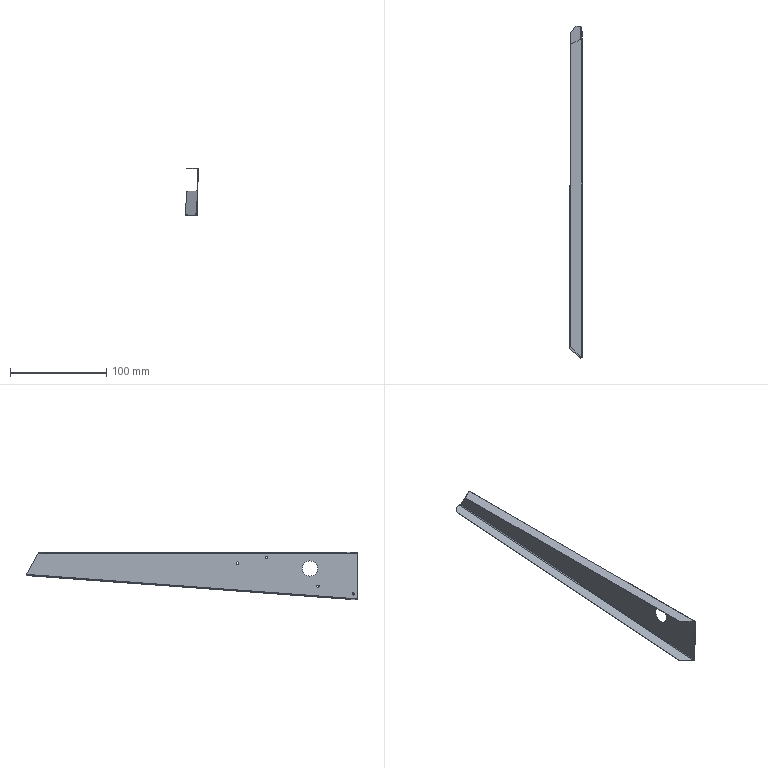Part | SolidWorks | features BaseBody 1 | 1 solid | 35 faces | box 13.154 x 345.624 x 49.869 mm | volume 9893 mm3 | plane 15 | cylinder 14 | spline 6 | commonest cylinder face diameters 2.4 x8 1.473 x2 2.473 x2 15.9 x2
STEP:
#1=CARTESIAN_POINT('',(-0.6458,-122.,-25.162));
#2=VERTEX_POINT('',#1);
#3=CARTESIAN_POINT('',(-0.2296,-122.,-9.267));
#4=VERTEX_POINT('',#3);
#5=CARTESIAN_POINT('',(-0.4377,-122.,-17.214));
#6=DIRECTION('',(-0.9997,0.,0.02618));
#7=DIRECTION('',(-0.02618,0.,-0.9997));
#8=AXIS2_PLACEMENT_3D('',#5,#6,#7);
#9=CIRCLE('',#8,7.95);
#10=EDGE_CURVE('',#2,#4,#9,.T.);
#11=ORIENTED_EDGE('',*,*,#10,.T.);
#12=CARTESIAN_POINT('',(0.2703,-122.,-9.28));
#13=VERTEX_POINT('',#12);
#14=CARTESIAN_POINT('',(-0.2296,-122.,-9.267));
#15=DIRECTION('',(0.9997,0.,-0.02618));
#16=VECTOR('',#15,1000.);
#17=LINE('',#14,#16);
#18=EDGE_CURVE('',#4,#13,#17,.T.);
#19=ORIENTED_EDGE('',*,*,#18,.T.);
#20=CARTESIAN_POINT('',(-0.146,-122.,-25.175));
#21=VERTEX_POINT('',#20);
#22=CARTESIAN_POINT('',(0.06215,-122.,-17.227));
#23=DIRECTION('',(0.9997,0.,-0.02618));
#24=DIRECTION('',(-0.02618,0.,-0.9997));
#25=AXIS2_PLACEMENT_3D('',#22,#23,#24);
#26=CIRCLE('',#25,7.95);
#27=EDGE_CURVE('',#13,#21,#26,.T.);
#28=ORIENTED_EDGE('',*,*,#27,.T.);
#29=CARTESIAN_POINT('',(-0.6458,-122.,-25.162));
#30=DIRECTION('',(0.9997,0.,-0.02618));
#31=VECTOR('',#30,1000.);
#32=LINE('',#29,#31);
#33=EDGE_CURVE('',#2,#21,#32,.T.);
#34=ORIENTED_EDGE('',*,*,#33,.F.);
#35=EDGE_LOOP('',(#11,#19,#28,#34));
#36=FACE_OUTER_BOUND('',#35,.T.);
#37=CARTESIAN_POINT('',(-0.4377,-122.,-17.214));
#38=DIRECTION('',(0.9997,0.,-0.02618));
#39=DIRECTION('',(-0.02618,0.,-0.9997));
#40=AXIS2_PLACEMENT_3D('',#37,#38,#39);
#41=CYLINDRICAL_SURFACE('',#40,7.95);
#42=ADVANCED_FACE('',(#36),#41,.F.);
#43=CARTESIAN_POINT('',(-0.3859,-130.324,-34.336));
#44=VERTEX_POINT('',#43);
#45=CARTESIAN_POINT('',(-0.4487,-130.324,-36.736));
#46=VERTEX_POINT('',#45);
#47=CARTESIAN_POINT('',(-0.4173,-130.324,-35.536));
#48=DIRECTION('',(0.9997,0.,-0.02618));
#49=DIRECTION('',(0.02618,0.,0.9997));
#50=AXIS2_PLACEMENT_3D('',#47,#48,#49);
#51=CIRCLE('',#50,1.2);
#52=EDGE_CURVE('',#44,#46,#51,.T.);
#53=ORIENTED_EDGE('',*,*,#52,.T.);
#54=CARTESIAN_POINT('',(-0.9485,-130.324,-36.723));
#55=VERTEX_POINT('',#54);
#56=CARTESIAN_POINT('',(-0.4487,-130.324,-36.736));
#57=DIRECTION('',(-0.9997,0.,0.02618));
#58=VECTOR('',#57,1000.);
#59=LINE('',#56,#58);
#60=EDGE_CURVE('',#46,#55,#59,.T.);
#61=ORIENTED_EDGE('',*,*,#60,.T.);
#62=CARTESIAN_POINT('',(-0.8857,-130.324,-34.323));
#63=VERTEX_POINT('',#62);
#64=CARTESIAN_POINT('',(-0.9171,-130.324,-35.523));
#65=DIRECTION('',(0.9997,0.,-0.02618));
#66=DIRECTION('',(0.02618,0.,0.9997));
#67=AXIS2_PLACEMENT_3D('',#64,#65,#66);
#68=CIRCLE('',#67,1.2);
#69=EDGE_CURVE('',#63,#55,#68,.T.);
#70=ORIENTED_EDGE('',*,*,#69,.F.);
#71=CARTESIAN_POINT('',(-0.3859,-130.324,-34.336));
#72=DIRECTION('',(-0.9997,0.,0.02618));
#73=VECTOR('',#72,1000.);
#74=LINE('',#71,#73);
#75=EDGE_CURVE('',#44,#63,#74,.T.);
#76=ORIENTED_EDGE('',*,*,#75,.F.);
#77=EDGE_LOOP('',(#53,#61,#70,#76));
#78=FACE_OUTER_BOUND('',#77,.T.);
#79=CARTESIAN_POINT('',(-0.4173,-130.324,-35.536));
#80=DIRECTION('',(-0.9997,0.,0.02618));
#81=DIRECTION('',(0.02618,0.,0.9997));
#82=AXIS2_PLACEMENT_3D('',#79,#80,#81);
#83=CYLINDRICAL_SURFACE('',#82,1.2);
#84=ADVANCED_FACE('',(#78),#83,.F.);
#85=CARTESIAN_POINT('',(-0.5954,-167.,-42.338));
#86=VERTEX_POINT('',#85);
#87=CARTESIAN_POINT('',(-0.6582,-167.,-44.738));
#88=VERTEX_POINT('',#87);
#89=CARTESIAN_POINT('',(-0.6268,-167.,-43.538));
#90=DIRECTION('',(0.9997,0.,-0.02618));
#91=DIRECTION('',(0.02618,0.,0.9997));
#92=AXIS2_PLACEMENT_3D('',#89,#90,#91);
#93=CIRCLE('',#92,1.2);
#94=EDGE_CURVE('',#86,#88,#93,.T.);
#95=ORIENTED_EDGE('',*,*,#94,.T.);
#96=CARTESIAN_POINT('',(-1.158,-167.,-44.724));
#97=VERTEX_POINT('',#96);
#98=CARTESIAN_POINT('',(-0.6582,-167.,-44.738));
#99=DIRECTION('',(-0.9997,0.,0.02618));
#100=VECTOR('',#99,1000.);
#101=LINE('',#98,#100);
#102=EDGE_CURVE('',#88,#97,#101,.T.);
#103=ORIENTED_EDGE('',*,*,#102,.T.);
#104=CARTESIAN_POINT('',(-1.095,-167.,-42.325));
#105=VERTEX_POINT('',#104);
#106=CARTESIAN_POINT('',(-1.127,-167.,-43.525));
#107=DIRECTION('',(0.9997,0.,-0.02618));
#108=DIRECTION('',(0.02618,0.,0.9997));
#109=AXIS2_PLACEMENT_3D('',#106,#107,#108);
#110=CIRCLE('',#109,1.2);
#111=EDGE_CURVE('',#105,#97,#110,.T.);
#112=ORIENTED_EDGE('',*,*,#111,.F.);
#113=CARTESIAN_POINT('',(-0.5954,-167.,-42.338));
#114=DIRECTION('',(-0.9997,0.,0.02618));
#115=VECTOR('',#114,1000.);
#116=LINE('',#113,#115);
#117=EDGE_CURVE('',#86,#105,#116,.T.);
#118=ORIENTED_EDGE('',*,*,#117,.F.);
#119=EDGE_LOOP('',(#95,#103,#112,#118));
#120=FACE_OUTER_BOUND('',#119,.T.);
#121=CARTESIAN_POINT('',(-0.6268,-167.,-43.538));
#122=DIRECTION('',(-0.9997,0.,0.02618));
#123=DIRECTION('',(0.02618,0.,0.9997));
#124=AXIS2_PLACEMENT_3D('',#121,#122,#123);
#125=CYLINDRICAL_SURFACE('',#124,1.2);
#126=ADVANCED_FACE('',(#120),#125,.F.);
#127=CARTESIAN_POINT('',(0.3873,-77.,-4.812));
#128=VERTEX_POINT('',#127);
#129=CARTESIAN_POINT('',(0.3244,-77.,-7.211));
#130=VERTEX_POINT('',#129);
#131=CARTESIAN_POINT('',(0.3559,-77.,-6.011));
#132=DIRECTION('',(0.9997,0.,-0.02618));
#133=DIRECTION('',(0.02618,0.,0.9997));
#134=AXIS2_PLACEMENT_3D('',#131,#132,#133);
#135=CIRCLE('',#134,1.2);
#136=EDGE_CURVE('',#128,#130,#135,.T.);
#137=ORIENTED_EDGE('',*,*,#136,.T.);
#138=CARTESIAN_POINT('',(-0.1754,-77.,-7.198));
#139=VERTEX_POINT('',#138);
#140=CARTESIAN_POINT('',(0.3244,-77.,-7.211));
#141=DIRECTION('',(-0.9997,0.,0.02618));
#142=VECTOR('',#141,1000.);
#143=LINE('',#140,#142);
#144=EDGE_CURVE('',#130,#139,#143,.T.);
#145=ORIENTED_EDGE('',*,*,#144,.T.);
#146=CARTESIAN_POINT('',(-0.1126,-77.,-4.799));
#147=VERTEX_POINT('',#146);
#148=CARTESIAN_POINT('',(-0.144,-77.,-5.998));
#149=DIRECTION('',(0.9997,0.,-0.02618));
#150=DIRECTION('',(0.02618,0.,0.9997));
#151=AXIS2_PLACEMENT_3D('',#148,#149,#150);
#152=CIRCLE('',#151,1.2);
#153=EDGE_CURVE('',#147,#139,#152,.T.);
#154=ORIENTED_EDGE('',*,*,#153,.F.);
#155=CARTESIAN_POINT('',(0.3873,-77.,-4.812));
#156=DIRECTION('',(-0.9997,0.,0.02618));
#157=VECTOR('',#156,1000.);
#158=LINE('',#155,#157);
#159=EDGE_CURVE('',#128,#147,#158,.T.);
#160=ORIENTED_EDGE('',*,*,#159,.F.);
#161=EDGE_LOOP('',(#137,#145,#154,#160));
#162=FACE_OUTER_BOUND('',#161,.T.);
#163=CARTESIAN_POINT('',(0.3559,-77.,-6.011));
#164=DIRECTION('',(-0.9997,0.,0.02618));
#165=DIRECTION('',(0.02618,0.,0.9997));
#166=AXIS2_PLACEMENT_3D('',#163,#164,#165);
#167=CYLINDRICAL_SURFACE('',#166,1.2);
#168=ADVANCED_FACE('',(#162),#167,.F.);
#169=CARTESIAN_POINT('',(0.2442,-46.588,-10.273));
#170=VERTEX_POINT('',#169);
#171=CARTESIAN_POINT('',(0.1814,-46.588,-12.672));
#172=VERTEX_POINT('',#171);
#173=CARTESIAN_POINT('',(0.2128,-46.588,-11.473));
#174=DIRECTION('',(0.9997,0.,-0.02618));
#175=DIRECTION('',(0.02618,0.,0.9997));
#176=AXIS2_PLACEMENT_3D('',#173,#174,#175);
#177=CIRCLE('',#176,1.2);
#178=EDGE_CURVE('',#170,#172,#177,.T.);
#179=ORIENTED_EDGE('',*,*,#178,.T.);
#180=CARTESIAN_POINT('',(-0.3184,-46.588,-12.659));
#181=VERTEX_POINT('',#180);
#182=CARTESIAN_POINT('',(0.1814,-46.588,-12.672));
#183=DIRECTION('',(-0.9997,0.,0.02618));
#184=VECTOR('',#183,1000.);
#185=LINE('',#182,#184);
#186=EDGE_CURVE('',#172,#181,#185,.T.);
#187=ORIENTED_EDGE('',*,*,#186,.T.);
#188=CARTESIAN_POINT('',(-0.2556,-46.588,-10.26));
#189=VERTEX_POINT('',#188);
#190=CARTESIAN_POINT('',(-0.287,-46.588,-11.46));
#191=DIRECTION('',(0.9997,0.,-0.02618));
#192=DIRECTION('',(0.02618,0.,0.9997));
#193=AXIS2_PLACEMENT_3D('',#190,#191,#192);
#194=CIRCLE('',#193,1.2);
#195=EDGE_CURVE('',#189,#181,#194,.T.);
#196=ORIENTED_EDGE('',*,*,#195,.F.);
#197=CARTESIAN_POINT('',(0.2442,-46.588,-10.273));
#198=DIRECTION('',(-0.9997,0.,0.02618));
#199=VECTOR('',#198,1000.);
#200=LINE('',#197,#199);
#201=EDGE_CURVE('',#170,#189,#200,.T.);
#202=ORIENTED_EDGE('',*,*,#201,.F.);
#203=EDGE_LOOP('',(#179,#187,#196,#202));
#204=FACE_OUTER_BOUND('',#203,.T.);
#205=CARTESIAN_POINT('',(0.2128,-46.588,-11.473));
#206=DIRECTION('',(-0.9997,0.,0.02618));
#207=DIRECTION('',(0.02618,0.,0.9997));
#208=AXIS2_PLACEMENT_3D('',#205,#206,#207);
#209=CYLINDRICAL_SURFACE('',#208,1.2);
#210=ADVANCED_FACE('',(#204),#209,.F.);
#211=ORIENTED_EDGE('',*,*,#18,.F.);
#212=CARTESIAN_POINT('',(-0.4377,-122.,-17.214));
#213=DIRECTION('',(-0.9997,0.,0.02618));
#214=DIRECTION('',(-0.02618,0.,-0.9997));
#215=AXIS2_PLACEMENT_3D('',#212,#213,#214);
#216=CIRCLE('',#215,7.95);
#217=EDGE_CURVE('',#4,#2,#216,.T.);
#218=ORIENTED_EDGE('',*,*,#217,.T.);
#219=ORIENTED_EDGE('',*,*,#33,.T.);
#220=CARTESIAN_POINT('',(0.06215,-122.,-17.227));
#221=DIRECTION('',(0.9997,0.,-0.02618));
#222=DIRECTION('',(-0.02618,0.,-0.9997));
#223=AXIS2_PLACEMENT_3D('',#220,#221,#222);
#224=CIRCLE('',#223,7.95);
#225=EDGE_CURVE('',#21,#13,#224,.T.);
#226=ORIENTED_EDGE('',*,*,#225,.T.);
#227=EDGE_LOOP('',(#211,#218,#219,#226));
#228=FACE_OUTER_BOUND('',#227,.T.);
#229=CARTESIAN_POINT('',(-0.4377,-122.,-17.214));
#230=DIRECTION('',(0.9997,0.,-0.02618));
#231=DIRECTION('',(-0.02618,0.,-0.9997));
#232=AXIS2_PLACEMENT_3D('',#229,#230,#231);
#233=CYLINDRICAL_SURFACE('',#232,7.95);
#234=ADVANCED_FACE('',(#228),#233,.F.);
#235=ORIENTED_EDGE('',*,*,#52,.F.);
#236=CARTESIAN_POINT('',(-0.4173,-130.324,-35.536));
#237=DIRECTION('',(0.9997,0.,-0.02618));
#238=DIRECTION('',(0.02618,0.,0.9997));
#239=AXIS2_PLACEMENT_3D('',#236,#237,#238);
#240=CIRCLE('',#239,1.2);
#241=EDGE_CURVE('',#46,#44,#240,.T.);
#242=ORIENTED_EDGE('',*,*,#241,.F.);
#243=EDGE_LOOP('',(#235,#242));
#244=FACE_BOUND('',#243,.T.);
#245=ORIENTED_EDGE('',*,*,#94,.F.);
#246=CARTESIAN_POINT('',(-0.6268,-167.,-43.538));
#247=DIRECTION('',(0.9997,0.,-0.02618));
#248=DIRECTION('',(0.02618,0.,0.9997));
#249=AXIS2_PLACEMENT_3D('',#246,#247,#248);
#250=CIRCLE('',#249,1.2);
#251=EDGE_CURVE('',#88,#86,#250,.T.);
#252=ORIENTED_EDGE('',*,*,#251,.F.);
#253=EDGE_LOOP('',(#245,#252));
#254=FACE_BOUND('',#253,.T.);
#255=ORIENTED_EDGE('',*,*,#136,.F.);
#256=CARTESIAN_POINT('',(0.3559,-77.,-6.011));
#257=DIRECTION('',(0.9997,0.,-0.02618));
#258=DIRECTION('',(0.02618,0.,0.9997));
#259=AXIS2_PLACEMENT_3D('',#256,#257,#258);
#260=CIRCLE('',#259,1.2);
#261=EDGE_CURVE('',#130,#128,#260,.T.);
#262=ORIENTED_EDGE('',*,*,#261,.F.);
#263=EDGE_LOOP('',(#255,#262));
#264=FACE_BOUND('',#263,.T.);
#265=ORIENTED_EDGE('',*,*,#178,.F.);
#266=CARTESIAN_POINT('',(0.2128,-46.588,-11.473));
#267=DIRECTION('',(0.9997,0.,-0.02618));
#268=DIRECTION('',(0.02618,0.,0.9997));
#269=AXIS2_PLACEMENT_3D('',#266,#267,#268);
#270=CIRCLE('',#269,1.2);
#271=EDGE_CURVE('',#172,#170,#270,.T.);
#272=ORIENTED_EDGE('',*,*,#271,.F.);
#273=EDGE_LOOP('',(#265,#272));
#274=FACE_BOUND('',#273,.T.);
#275=ORIENTED_EDGE('',*,*,#225,.F.);
#276=ORIENTED_EDGE('',*,*,#27,.F.);
#277=EDGE_LOOP('',(#275,#276));
#278=FACE_BOUND('',#277,.T.);
#279=CARTESIAN_POINT('',(0.48,-172.,-1.269));
#280=VERTEX_POINT('',#279);
#281=CARTESIAN_POINT('',(0.48,161.053,-1.269));
#282=VERTEX_POINT('',#281);
#283=CARTESIAN_POINT('',(0.48,1.644,-1.269));
#284=DIRECTION('',(0.,1.,0.));
#285=VECTOR('',#284,1000.);
#286=LINE('',#283,#285);
#287=EDGE_CURVE('',#280,#282,#286,.T.);
#288=ORIENTED_EDGE('',*,*,#287,.F.);
#289=CARTESIAN_POINT('',(-0.7624,-172.,-48.714));
#290=VERTEX_POINT('',#289);
#291=CARTESIAN_POINT('',(-0.1449,-172.,-25.134));
#292=DIRECTION('',(0.02618,0.,0.9997));
#293=VECTOR('',#292,1000.);
#294=LINE('',#291,#293);
#295=EDGE_CURVE('',#290,#280,#294,.T.);
#296=ORIENTED_EDGE('',*,*,#295,.F.);
#297=CARTESIAN_POINT('',(-0.09558,173.218,-23.251));
#298=VERTEX_POINT('',#297);
#299=CARTESIAN_POINT('',(-0.7665,-174.126,-48.871));
#300=DIRECTION('',(-0.001926,-0.9973,-0.07356));
#301=VECTOR('',#300,1000.);
#302=LINE('',#299,#301);
#303=EDGE_CURVE('',#298,#290,#302,.T.);
#304=ORIENTED_EDGE('',*,*,#303,.F.);
#305=CARTESIAN_POINT('',(0.48,161.053,-1.269));
#306=DIRECTION('',(-0.02291,0.4841,-0.8747));
#307=VECTOR('',#306,1000.);
#308=LINE('',#305,#307);
#309=EDGE_CURVE('',#282,#298,#308,.T.);
#310=ORIENTED_EDGE('',*,*,#309,.F.);
#311=EDGE_LOOP('',(#288,#296,#304,#310));
#312=FACE_OUTER_BOUND('',#311,.T.);
#313=CARTESIAN_POINT('',(0.48,175.289,-1.269));
#314=DIRECTION('',(-0.9997,0.,0.02618));
#315=DIRECTION('',(-0.02618,0.,-0.9997));
#316=AXIS2_PLACEMENT_3D('',#313,#314,#315);
#317=PLANE('',#316);
#318=ADVANCED_FACE('',(#244,#254,#264,#274,#278,#312),#317,.F.);
#319=ORIENTED_EDGE('',*,*,#69,.T.);
#320=CARTESIAN_POINT('',(-0.9171,-130.324,-35.523));
#321=DIRECTION('',(0.9997,0.,-0.02618));
#322=DIRECTION('',(0.02618,0.,0.9997));
#323=AXIS2_PLACEMENT_3D('',#320,#321,#322);
#324=CIRCLE('',#323,1.2);
#325=EDGE_CURVE('',#55,#63,#324,.T.);
#326=ORIENTED_EDGE('',*,*,#325,.T.);
#327=EDGE_LOOP('',(#319,#326));
#328=FACE_BOUND('',#327,.T.);
#329=ORIENTED_EDGE('',*,*,#111,.T.);
#330=CARTESIAN_POINT('',(-1.127,-167.,-43.525));
#331=DIRECTION('',(0.9997,0.,-0.02618));
#332=DIRECTION('',(0.02618,0.,0.9997));
#333=AXIS2_PLACEMENT_3D('',#330,#331,#332);
#334=CIRCLE('',#333,1.2);
#335=EDGE_CURVE('',#97,#105,#334,.T.);
#336=ORIENTED_EDGE('',*,*,#335,.T.);
#337=EDGE_LOOP('',(#329,#336));
#338=FACE_BOUND('',#337,.T.);
#339=ORIENTED_EDGE('',*,*,#153,.T.);
#340=CARTESIAN_POINT('',(-0.144,-77.,-5.998));
#341=DIRECTION('',(0.9997,0.,-0.02618));
#342=DIRECTION('',(0.02618,0.,0.9997));
#343=AXIS2_PLACEMENT_3D('',#340,#341,#342);
#344=CIRCLE('',#343,1.2);
#345=EDGE_CURVE('',#139,#147,#344,.T.);
#346=ORIENTED_EDGE('',*,*,#345,.T.);
#347=EDGE_LOOP('',(#339,#346));
#348=FACE_BOUND('',#347,.T.);
#349=ORIENTED_EDGE('',*,*,#195,.T.);
#350=CARTESIAN_POINT('',(-0.287,-46.588,-11.46));
#351=DIRECTION('',(0.9997,0.,-0.02618));
#352=DIRECTION('',(0.02618,0.,0.9997));
#353=AXIS2_PLACEMENT_3D('',#350,#351,#352);
#354=CIRCLE('',#353,1.2);
#355=EDGE_CURVE('',#181,#189,#354,.T.);
#356=ORIENTED_EDGE('',*,*,#355,.T.);
#357=EDGE_LOOP('',(#349,#356));
#358=FACE_BOUND('',#357,.T.);
#359=ORIENTED_EDGE('',*,*,#10,.F.);
#360=ORIENTED_EDGE('',*,*,#217,.F.);
#361=EDGE_LOOP('',(#359,#360));
#362=FACE_BOUND('',#361,.T.);
#363=CARTESIAN_POINT('',(-0.01979,-172.,-1.256));
#364=VERTEX_POINT('',#363);
#365=CARTESIAN_POINT('',(-0.01979,161.053,-1.256));
#366=VERTEX_POINT('',#365);
#367=CARTESIAN_POINT('',(-0.01979,1.644,-1.256));
#368=DIRECTION('',(0.,1.,0.));
#369=VECTOR('',#368,1000.);
#370=LINE('',#367,#369);
#371=EDGE_CURVE('',#364,#366,#370,.T.);
#372=ORIENTED_EDGE('',*,*,#371,.T.);
#373=CARTESIAN_POINT('',(-0.5954,173.218,-23.238));
#374=VERTEX_POINT('',#373);
#375=CARTESIAN_POINT('',(-0.01979,161.053,-1.256));
#376=DIRECTION('',(-0.02291,0.4841,-0.8747));
#377=VECTOR('',#376,1000.);
#378=LINE('',#375,#377);
#379=EDGE_CURVE('',#366,#374,#378,.T.);
#380=ORIENTED_EDGE('',*,*,#379,.T.);
#381=CARTESIAN_POINT('',(-1.262,-172.,-48.701));
#382=VERTEX_POINT('',#381);
#383=CARTESIAN_POINT('',(-0.5954,173.218,-23.238));
#384=DIRECTION('',(-0.001926,-0.9973,-0.07356));
#385=VECTOR('',#384,1000.);
#386=LINE('',#383,#385);
#387=EDGE_CURVE('',#374,#382,#386,.T.);
#388=ORIENTED_EDGE('',*,*,#387,.T.);
#389=CARTESIAN_POINT('',(-0.6447,-172.,-25.121));
#390=DIRECTION('',(0.02618,0.,0.9997));
#391=VECTOR('',#390,1000.);
#392=LINE('',#389,#391);
#393=EDGE_CURVE('',#382,#364,#392,.T.);
#394=ORIENTED_EDGE('',*,*,#393,.T.);
#395=EDGE_LOOP('',(#372,#380,#388,#394));
#396=FACE_OUTER_BOUND('',#395,.T.);
#397=CARTESIAN_POINT('',(-0.01979,175.289,-1.256));
#398=DIRECTION('',(-0.9997,0.,0.02618));
#399=DIRECTION('',(-0.02618,0.,-0.9997));
#400=AXIS2_PLACEMENT_3D('',#397,#398,#399);
#401=PLANE('',#400);
#402=ADVANCED_FACE('',(#328,#338,#348,#358,#362,#396),#401,.T.);
#403=ORIENTED_EDGE('',*,*,#60,.F.);
#404=ORIENTED_EDGE('',*,*,#241,.T.);
#405=ORIENTED_EDGE('',*,*,#75,.T.);
#406=ORIENTED_EDGE('',*,*,#325,.F.);
#407=EDGE_LOOP('',(#403,#404,#405,#406));
#408=FACE_OUTER_BOUND('',#407,.T.);
#409=CARTESIAN_POINT('',(-0.4173,-130.324,-35.536));
#410=DIRECTION('',(-0.9997,0.,0.02618));
#411=DIRECTION('',(0.02618,0.,0.9997));
#412=AXIS2_PLACEMENT_3D('',#409,#410,#411);
#413=CYLINDRICAL_SURFACE('',#412,1.2);
#414=ADVANCED_FACE('',(#408),#413,.F.);
#415=ORIENTED_EDGE('',*,*,#102,.F.);
#416=ORIENTED_EDGE('',*,*,#251,.T.);
#417=ORIENTED_EDGE('',*,*,#117,.T.);
#418=ORIENTED_EDGE('',*,*,#335,.F.);
#419=EDGE_LOOP('',(#415,#416,#417,#418));
#420=FACE_OUTER_BOUND('',#419,.T.);
#421=CARTESIAN_POINT('',(-0.6268,-167.,-43.538));
#422=DIRECTION('',(-0.9997,0.,0.02618));
#423=DIRECTION('',(0.02618,0.,0.9997));
#424=AXIS2_PLACEMENT_3D('',#421,#422,#423);
#425=CYLINDRICAL_SURFACE('',#424,1.2);
#426=ADVANCED_FACE('',(#420),#425,.F.);
#427=ORIENTED_EDGE('',*,*,#144,.F.);
#428=ORIENTED_EDGE('',*,*,#261,.T.);
#429=ORIENTED_EDGE('',*,*,#159,.T.);
#430=ORIENTED_EDGE('',*,*,#345,.F.);
#431=EDGE_LOOP('',(#427,#428,#429,#430));
#432=FACE_OUTER_BOUND('',#431,.T.);
#433=CARTESIAN_POINT('',(0.3559,-77.,-6.011));
#434=DIRECTION('',(-0.9997,0.,0.02618));
#435=DIRECTION('',(0.02618,0.,0.9997));
#436=AXIS2_PLACEMENT_3D('',#433,#434,#435);
#437=CYLINDRICAL_SURFACE('',#436,1.2);
#438=ADVANCED_FACE('',(#432),#437,.F.);
#439=ORIENTED_EDGE('',*,*,#186,.F.);
#440=ORIENTED_EDGE('',*,*,#271,.T.);
#441=ORIENTED_EDGE('',*,*,#201,.T.);
#442=ORIENTED_EDGE('',*,*,#355,.F.);
#443=EDGE_LOOP('',(#439,#440,#441,#442));
#444=FACE_OUTER_BOUND('',#443,.T.);
#445=CARTESIAN_POINT('',(0.2128,-46.588,-11.473));
#446=DIRECTION('',(-0.9997,0.,0.02618));
#447=DIRECTION('',(0.02618,0.,0.9997));
#448=AXIS2_PLACEMENT_3D('',#445,#446,#447);
#449=CYLINDRICAL_SURFACE('',#448,1.2);
#450=ADVANCED_FACE('',(#444),#449,.F.);
#451=CARTESIAN_POINT('',(0.2301,161.053,-1.262));
#452=DIRECTION('',(-0.9997,0.,0.02618));
#453=VECTOR('',#452,1000.);
#454=LINE('',#451,#453);
#455=EDGE_CURVE('',#282,#366,#454,.T.);
#456=ORIENTED_EDGE('',*,*,#455,.F.);
#457=ORIENTED_EDGE('',*,*,#309,.T.);
#458=CARTESIAN_POINT('',(-0.3455,173.218,-23.244));
#459=DIRECTION('',(0.9997,0.,-0.02618));
#460=VECTOR('',#459,1000.);
#461=LINE('',#458,#460);
#462=EDGE_CURVE('',#374,#298,#461,.T.);
#463=ORIENTED_EDGE('',*,*,#462,.F.);
#464=ORIENTED_EDGE('',*,*,#379,.F.);
#465=EDGE_LOOP('',(#456,#457,#463,#464));
#466=FACE_OUTER_BOUND('',#465,.T.);
#467=CARTESIAN_POINT('',(-0.01979,161.053,-1.256));
#468=DIRECTION('',(-0.01267,-0.875,-0.4839));
#469=DIRECTION('',(-0.02291,0.4841,-0.8747));
#470=AXIS2_PLACEMENT_3D('',#467,#468,#469);
#471=PLANE('',#470);
#472=ADVANCED_FACE('',(#466),#471,.F.);
#473=CARTESIAN_POINT('',(0.1015,-172.,-0.3457));
#474=VERTEX_POINT('',#473);
#475=CARTESIAN_POINT('',(-0.7561,-172.,-1.237));
#476=DIRECTION('',(0.,-1.,0.));
#477=DIRECTION('',(0.,0.,1.));
#478=AXIS2_PLACEMENT_3D('',#475,#476,#477);
#479=CIRCLE('',#478,1.237);
#480=EDGE_CURVE('',#280,#474,#479,.T.);
#481=ORIENTED_EDGE('',*,*,#480,.F.);
#482=ORIENTED_EDGE('',*,*,#287,.T.);
#483=CARTESIAN_POINT('',(-0.7561,160.182,0.));
#484=VERTEX_POINT('',#483);
#485=CARTESIAN_POINT('',(-0.7561,160.182,0.));
#486=CARTESIAN_POINT('',(-0.5901,160.255,0.000000001));
#487=CARTESIAN_POINT('',(-0.4278,160.327,-0.03298));
#488=CARTESIAN_POINT('',(-0.1232,160.473,-0.1615));
#489=CARTESIAN_POINT('',(0.0145,160.545,-0.2556));
#490=CARTESIAN_POINT('',(0.3594,160.763,-0.6095));
#491=CARTESIAN_POINT('',(0.4887,160.907,-0.937));
#492=CARTESIAN_POINT('',(0.48,161.053,-1.269));
#493=B_SPLINE_CURVE_WITH_KNOTS('',3,(#485,#486,#487,#488,#489,#490,#491,#492),.UNSPECIFIED.,.F.,.F.,(4,2,2,4),(0.,0.0005368,0.001074,0.002147),.UNSPECIFIED.);
#494=EDGE_CURVE('',#484,#282,#493,.T.);
#495=ORIENTED_EDGE('',*,*,#494,.F.);
#496=CARTESIAN_POINT('',(-0.7561,-171.244,0.));
#497=VERTEX_POINT('',#496);
#498=CARTESIAN_POINT('',(-0.7561,-4.474,0.));
#499=DIRECTION('',(0.,1.,0.));
#500=VECTOR('',#499,1000.);
#501=LINE('',#498,#500);
#502=EDGE_CURVE('',#497,#484,#501,.T.);
#503=ORIENTED_EDGE('',*,*,#502,.F.);
#504=CARTESIAN_POINT('',(0.1015,-172.,-0.3457));
#505=CARTESIAN_POINT('',(-0.01273,-171.873,-0.2358));
#506=CARTESIAN_POINT('',(-0.1476,-171.748,-0.1485));
#507=CARTESIAN_POINT('',(-0.4412,-171.495,-0.03035));
#508=CARTESIAN_POINT('',(-0.5976,-171.37,0.000000004));
#509=CARTESIAN_POINT('',(-0.7561,-171.244,0.));
#510=B_SPLINE_CURVE_WITH_KNOTS('',3,(#504,#505,#506,#507,#508,#509),.UNSPECIFIED.,.F.,.F.,(4,2,4),(0.,0.0006065,0.001213),.UNSPECIFIED.);
#511=EDGE_CURVE('',#474,#497,#510,.T.);
#512=ORIENTED_EDGE('',*,*,#511,.F.);
#513=EDGE_LOOP('',(#481,#482,#495,#503,#512));
#514=FACE_OUTER_BOUND('',#513,.T.);
#515=CARTESIAN_POINT('',(-0.7561,-172.,-1.237));
#516=DIRECTION('',(0.,1.,0.));
#517=DIRECTION('',(0.,0.,1.));
#518=AXIS2_PLACEMENT_3D('',#515,#516,#517);
#519=CYLINDRICAL_SURFACE('',#518,1.237);
#520=ADVANCED_FACE('',(#514),#519,.T.);
#521=ORIENTED_EDGE('',*,*,#295,.T.);
#522=ORIENTED_EDGE('',*,*,#480,.T.);
#523=CARTESIAN_POINT('',(-0.2453,-172.,-0.706));
#524=VERTEX_POINT('',#523);
#525=CARTESIAN_POINT('',(-0.07188,-172.,-0.5258));
#526=DIRECTION('',(0.6936,0.,0.7204));
#527=VECTOR('',#526,1000.);
#528=LINE('',#525,#527);
#529=EDGE_CURVE('',#524,#474,#528,.T.);
#530=ORIENTED_EDGE('',*,*,#529,.F.);
#531=CARTESIAN_POINT('',(-0.7561,-172.,-1.237));
#532=DIRECTION('',(0.,-1.,0.));
#533=DIRECTION('',(0.,0.,1.));
#534=AXIS2_PLACEMENT_3D('',#531,#532,#533);
#535=CIRCLE('',#534,0.7366);
#536=EDGE_CURVE('',#364,#524,#535,.T.);
#537=ORIENTED_EDGE('',*,*,#536,.F.);
#538=ORIENTED_EDGE('',*,*,#393,.F.);
#539=CARTESIAN_POINT('',(-1.012,-172.,-48.707));
#540=DIRECTION('',(-0.9997,0.,0.02618));
#541=VECTOR('',#540,1000.);
#542=LINE('',#539,#541);
#543=EDGE_CURVE('',#290,#382,#542,.T.);
#544=ORIENTED_EDGE('',*,*,#543,.F.);
#545=EDGE_LOOP('',(#521,#522,#530,#537,#538,#544));
#546=FACE_OUTER_BOUND('',#545,.T.);
#547=CARTESIAN_POINT('',(-0.7624,-172.,-48.714));
#548=DIRECTION('',(0.,1.,0.));
#549=DIRECTION('',(-0.9997,0.,0.02618));
#550=AXIS2_PLACEMENT_3D('',#547,#548,#549);
#551=PLANE('',#550);
#552=ADVANCED_FACE('',(#546),#551,.F.);
#553=CARTESIAN_POINT('',(-1.997,-171.268,-49.867));
#554=VERTEX_POINT('',#553);
#555=CARTESIAN_POINT('',(-1.097,-171.992,-49.529));
#556=VERTEX_POINT('',#555);
#557=CARTESIAN_POINT('',(-1.997,-171.268,-49.867));
#558=CARTESIAN_POINT('',(-1.828,-171.385,-49.876));
#559=CARTESIAN_POINT('',(-1.662,-171.502,-49.85));
#560=CARTESIAN_POINT('',(-1.352,-171.744,-49.733));
#561=CARTESIAN_POINT('',(-1.212,-171.867,-49.644));
#562=CARTESIAN_POINT('',(-1.097,-171.992,-49.529));
#563=B_SPLINE_CURVE_WITH_KNOTS('',3,(#557,#558,#559,#560,#561,#562),.UNSPECIFIED.,.F.,.F.,(4,2,4),(0.,0.0006103,0.001221),.UNSPECIFIED.);
#564=EDGE_CURVE('',#554,#556,#563,.T.);
#565=ORIENTED_EDGE('',*,*,#564,.F.);
#566=CARTESIAN_POINT('',(-1.331,173.579,-24.432));
#567=VERTEX_POINT('',#566);
#568=CARTESIAN_POINT('',(-1.665,0.8382,-37.173));
#569=DIRECTION('',(-0.001926,-0.9973,-0.07356));
#570=VECTOR('',#569,1000.);
#571=LINE('',#568,#570);
#572=EDGE_CURVE('',#567,#554,#571,.T.);
#573=ORIENTED_EDGE('',*,*,#572,.F.);
#574=CARTESIAN_POINT('',(-0.4292,173.608,-24.038));
#575=VERTEX_POINT('',#574);
#576=CARTESIAN_POINT('',(-0.4292,173.608,-24.038));
#577=CARTESIAN_POINT('',(-0.4873,173.607,-24.1));
#578=CARTESIAN_POINT('',(-0.5507,173.607,-24.155));
#579=CARTESIAN_POINT('',(-0.6877,173.604,-24.252));
#580=CARTESIAN_POINT('',(-0.7622,173.602,-24.294));
#581=CARTESIAN_POINT('',(-0.9938,173.595,-24.395));
#582=CARTESIAN_POINT('',(-1.161,173.588,-24.431));
#583=CARTESIAN_POINT('',(-1.331,173.579,-24.432));
#584=B_SPLINE_CURVE_WITH_KNOTS('',3,(#576,#577,#578,#579,#580,#581,#582,#583),.UNSPECIFIED.,.F.,.F.,(4,2,2,4),(0.,0.0002516,0.0005031,0.001006),.UNSPECIFIED.);
#585=EDGE_CURVE('',#575,#567,#584,.T.);
#586=ORIENTED_EDGE('',*,*,#585,.F.);
#587=CARTESIAN_POINT('',(-0.09558,173.218,-23.251));
#588=CARTESIAN_POINT('',(-0.1032,173.35,-23.541));
#589=CARTESIAN_POINT('',(-0.2243,173.481,-23.828));
#590=CARTESIAN_POINT('',(-0.4292,173.608,-24.038));
#591=B_SPLINE_CURVE_WITH_KNOTS('',3,(#587,#588,#589,#590),.UNSPECIFIED.,.F.,.F.,(4,4),(0.,1.),.UNSPECIFIED.);
#592=EDGE_CURVE('',#298,#575,#591,.T.);
#593=ORIENTED_EDGE('',*,*,#592,.F.);
#594=ORIENTED_EDGE('',*,*,#303,.T.);
#595=CARTESIAN_POINT('',(-1.097,-171.992,-49.529));
#596=CARTESIAN_POINT('',(-0.8916,-171.991,-49.31));
#597=CARTESIAN_POINT('',(-0.7702,-171.996,-49.014));
#598=CARTESIAN_POINT('',(-0.7624,-172.,-48.714));
#599=B_SPLINE_CURVE_WITH_KNOTS('',3,(#595,#596,#597,#598),.UNSPECIFIED.,.F.,.F.,(4,4),(0.,1.),.UNSPECIFIED.);
#600=EDGE_CURVE('',#556,#290,#599,.T.);
#601=ORIENTED_EDGE('',*,*,#600,.F.);
#602=EDGE_LOOP('',(#565,#573,#586,#593,#594,#601));
#603=FACE_OUTER_BOUND('',#602,.T.);
#604=CARTESIAN_POINT('',(-2.003,-174.126,-48.838));
#605=DIRECTION('',(0.001926,0.9973,0.07356));
#606=DIRECTION('',(0.,-0.07356,0.9973));
#607=AXIS2_PLACEMENT_3D('',#604,#605,#606);
#608=CYLINDRICAL_SURFACE('',#607,1.237);
#609=ADVANCED_FACE('',(#603),#608,.T.);
#610=ORIENTED_EDGE('',*,*,#371,.F.);
#611=ORIENTED_EDGE('',*,*,#536,.T.);
#612=CARTESIAN_POINT('',(-0.7561,-171.244,-0.5));
#613=VERTEX_POINT('',#612);
#614=CARTESIAN_POINT('',(-0.2453,-172.,-0.706));
#615=CARTESIAN_POINT('',(-0.2636,-171.966,-0.6883));
#616=CARTESIAN_POINT('',(-0.2828,-171.932,-0.6717));
#617=CARTESIAN_POINT('',(-0.3028,-171.898,-0.656));
#618=CARTESIAN_POINT('',(-0.3228,-171.864,-0.6404));
#619=CARTESIAN_POINT('',(-0.3436,-171.83,-0.6258));
#620=CARTESIAN_POINT('',(-0.3652,-171.796,-0.6123));
#621=CARTESIAN_POINT('',(-0.3867,-171.762,-0.5989));
#622=CARTESIAN_POINT('',(-0.4089,-171.728,-0.5865));
#623=CARTESIAN_POINT('',(-0.4317,-171.694,-0.5753));
#624=CARTESIAN_POINT('',(-0.4545,-171.66,-0.5641));
#625=CARTESIAN_POINT('',(-0.4779,-171.626,-0.5541));
#626=CARTESIAN_POINT('',(-0.5017,-171.592,-0.5453));
#627=CARTESIAN_POINT('',(-0.5256,-171.558,-0.5366));
#628=CARTESIAN_POINT('',(-0.5498,-171.524,-0.529));
#629=CARTESIAN_POINT('',(-0.5745,-171.49,-0.5228));
#630=CARTESIAN_POINT('',(-0.5991,-171.456,-0.5165));
#631=CARTESIAN_POINT('',(-0.624,-171.422,-0.5115));
#632=CARTESIAN_POINT('',(-0.6491,-171.388,-0.5078));
#633=CARTESIAN_POINT('',(-0.6668,-171.364,-0.5052));
#634=CARTESIAN_POINT('',(-0.6846,-171.34,-0.5033));
#635=CARTESIAN_POINT('',(-0.7024,-171.316,-0.502));
#636=CARTESIAN_POINT('',(-0.7203,-171.292,-0.5007));
#637=CARTESIAN_POINT('',(-0.7382,-171.268,-0.5));
#638=CARTESIAN_POINT('',(-0.7561,-171.244,-0.5));
#639=B_SPLINE_CURVE_WITH_KNOTS('',3,(#614,#615,#616,#617,#618,#619,#620,#621,#622,#623,#624,#625,#626,#627,#628,#629,#630,#631,#632,#633,#634,#635,#636,#637,#638),.UNSPECIFIED.,.F.,.F.,(4,3,3,3,3,3,3,3,4),(0.,0.0001273,0.0002547,0.000382,0.0005093,0.0006367,0.000764,0.0008537,0.0009435),.UNSPECIFIED.);
#640=EDGE_CURVE('',#524,#613,#639,.T.);
#641=ORIENTED_EDGE('',*,*,#640,.T.);
#642=CARTESIAN_POINT('',(-0.7561,160.182,-0.5));
#643=VERTEX_POINT('',#642);
#644=CARTESIAN_POINT('',(-0.7561,-4.474,-0.5));
#645=DIRECTION('',(0.,1.,0.));
#646=VECTOR('',#645,1000.);
#647=LINE('',#644,#646);
#648=EDGE_CURVE('',#613,#643,#647,.T.);
#649=ORIENTED_EDGE('',*,*,#648,.T.);
#650=CARTESIAN_POINT('',(-0.7561,160.182,-0.5));
#651=CARTESIAN_POINT('',(-0.5584,160.328,-0.5));
#652=CARTESIAN_POINT('',(-0.3664,160.471,-0.5813));
#653=CARTESIAN_POINT('',(-0.09155,160.763,-0.863));
#654=CARTESIAN_POINT('',(-0.01462,160.907,-1.058));
#655=CARTESIAN_POINT('',(-0.01979,161.053,-1.256));
#656=B_SPLINE_CURVE_WITH_KNOTS('',3,(#650,#651,#652,#653,#654,#655),.UNSPECIFIED.,.F.,.F.,(4,2,4),(0.,0.000728,0.001456),.UNSPECIFIED.);
#657=EDGE_CURVE('',#643,#366,#656,.T.);
#658=ORIENTED_EDGE('',*,*,#657,.T.);
#659=EDGE_LOOP('',(#610,#611,#641,#649,#658));
#660=FACE_OUTER_BOUND('',#659,.T.);
#661=CARTESIAN_POINT('',(-0.7561,-172.,-1.237));
#662=DIRECTION('',(0.,1.,0.));
#663=DIRECTION('',(0.,0.,1.));
#664=AXIS2_PLACEMENT_3D('',#661,#662,#663);
#665=CYLINDRICAL_SURFACE('',#664,0.7366);
#666=ADVANCED_FACE('',(#660),#665,.F.);
#667=CARTESIAN_POINT('',(-1.331,173.542,-23.933));
#668=VERTEX_POINT('',#667);
#669=CARTESIAN_POINT('',(-1.997,-171.305,-49.369));
#670=VERTEX_POINT('',#669);
#671=CARTESIAN_POINT('',(-1.665,0.8014,-36.674));
#672=DIRECTION('',(-0.001926,-0.9973,-0.07356));
#673=VECTOR('',#672,1000.);
#674=LINE('',#671,#673);
#675=EDGE_CURVE('',#668,#670,#674,.T.);
#676=ORIENTED_EDGE('',*,*,#675,.T.);
#677=CARTESIAN_POINT('',(-1.461,-172.017,-49.188));
#678=VERTEX_POINT('',#677);
#679=CARTESIAN_POINT('',(-1.997,-171.305,-49.369));
#680=CARTESIAN_POINT('',(-1.797,-171.537,-49.386));
#681=CARTESIAN_POINT('',(-1.598,-171.774,-49.317));
#682=CARTESIAN_POINT('',(-1.461,-172.017,-49.188));
#683=B_SPLINE_CURVE_WITH_KNOTS('',3,(#679,#680,#681,#682),.UNSPECIFIED.,.F.,.F.,(4,4),(0.,0.0009206),.UNSPECIFIED.);
#684=EDGE_CURVE('',#670,#678,#683,.T.);
#685=ORIENTED_EDGE('',*,*,#684,.T.);
#686=CARTESIAN_POINT('',(-1.461,-172.017,-49.188));
#687=CARTESIAN_POINT('',(-1.339,-172.009,-49.057));
#688=CARTESIAN_POINT('',(-1.267,-172.004,-48.88));
#689=CARTESIAN_POINT('',(-1.262,-172.,-48.701));
#690=B_SPLINE_CURVE_WITH_KNOTS('',3,(#686,#687,#688,#689),.UNSPECIFIED.,.F.,.F.,(4,4),(0.,1.),.UNSPECIFIED.);
#691=EDGE_CURVE('',#678,#382,#690,.T.);
#692=ORIENTED_EDGE('',*,*,#691,.T.);
#693=ORIENTED_EDGE('',*,*,#387,.F.);
#694=CARTESIAN_POINT('',(-0.7939,173.583,-23.697));
#695=VERTEX_POINT('',#694);
#696=CARTESIAN_POINT('',(-0.5954,173.218,-23.238));
#697=CARTESIAN_POINT('',(-0.5999,173.341,-23.408));
#698=CARTESIAN_POINT('',(-0.6719,173.464,-23.575));
#699=CARTESIAN_POINT('',(-0.7939,173.583,-23.697));
#700=B_SPLINE_CURVE_WITH_KNOTS('',3,(#696,#697,#698,#699),.UNSPECIFIED.,.F.,.F.,(4,4),(0.,1.),.UNSPECIFIED.);
#701=EDGE_CURVE('',#374,#695,#700,.T.);
#702=ORIENTED_EDGE('',*,*,#701,.T.);
#703=CARTESIAN_POINT('',(-0.7939,173.583,-23.697));
#704=CARTESIAN_POINT('',(-0.9312,173.574,-23.844));
#705=CARTESIAN_POINT('',(-1.13,173.561,-23.932));
#706=CARTESIAN_POINT('',(-1.331,173.542,-23.933));
#707=B_SPLINE_CURVE_WITH_KNOTS('',3,(#703,#704,#705,#706),.UNSPECIFIED.,.F.,.F.,(4,4),(0.,1.),.UNSPECIFIED.);
#708=EDGE_CURVE('',#695,#668,#707,.T.);
#709=ORIENTED_EDGE('',*,*,#708,.T.);
#710=EDGE_LOOP('',(#676,#685,#692,#693,#702,#709));
#711=FACE_OUTER_BOUND('',#710,.T.);
#712=CARTESIAN_POINT('',(-2.003,-174.126,-48.838));
#713=DIRECTION('',(0.001926,0.9973,0.07356));
#714=DIRECTION('',(0.,-0.07356,0.9973));
#715=AXIS2_PLACEMENT_3D('',#712,#713,#714);
#716=CYLINDRICAL_SURFACE('',#715,0.7366);
#717=ADVANCED_FACE('',(#711),#716,.F.);
#718=ORIENTED_EDGE('',*,*,#462,.T.);
#719=ORIENTED_EDGE('',*,*,#592,.T.);
#720=CARTESIAN_POINT('',(-0.6115,173.595,-23.867));
#721=DIRECTION('',(-0.7294,-0.04892,0.6824));
#722=VECTOR('',#721,1000.);
#723=LINE('',#720,#722);
#724=EDGE_CURVE('',#575,#695,#723,.T.);
#725=ORIENTED_EDGE('',*,*,#724,.T.);
#726=ORIENTED_EDGE('',*,*,#701,.F.);
#727=EDGE_LOOP('',(#718,#719,#725,#726));
#728=FACE_OUTER_BOUND('',#727,.T.);
#729=CARTESIAN_POINT('',(-0.4292,173.608,-24.038));
#730=CARTESIAN_POINT('',(-0.3267,173.545,-23.933));
#731=CARTESIAN_POINT('',(-0.2444,173.48,-23.809));
#732=CARTESIAN_POINT('',(-0.1307,173.35,-23.541));
#733=CARTESIAN_POINT('',(-0.09938,173.284,-23.396));
#734=CARTESIAN_POINT('',(-0.09558,173.218,-23.251));
#735=CARTESIAN_POINT('',(-0.7939,173.583,-23.697));
#736=CARTESIAN_POINT('',(-0.7329,173.523,-23.636));
#737=CARTESIAN_POINT('',(-0.6839,173.463,-23.564));
#738=CARTESIAN_POINT('',(-0.6163,173.341,-23.407));
#739=CARTESIAN_POINT('',(-0.5976,173.279,-23.323));
#740=CARTESIAN_POINT('',(-0.5954,173.218,-23.238));
#741=CARTESIAN_POINT('',(-0.7975,173.583,-23.693));
#742=CARTESIAN_POINT('',(-0.737,173.523,-23.633));
#743=CARTESIAN_POINT('',(-0.6883,173.463,-23.561));
#744=CARTESIAN_POINT('',(-0.6211,173.341,-23.406));
#745=CARTESIAN_POINT('',(-0.6026,173.279,-23.322));
#746=CARTESIAN_POINT('',(-0.6004,173.218,-23.237));
#747=B_SPLINE_SURFACE_WITH_KNOTS('',1,3,((#729,#730,#731,#732,#733,#734),(#735,#736,#737,#738,#739,#740),(#741,#742,#743,#744,#745,#746)),.UNSPECIFIED.,.F.,.F.,.F.,(2,1,2),(4,2,4),(0.,1.,1.01),(0.,0.5,1.),.UNSPECIFIED.);
#748=ADVANCED_FACE('',(#728),#747,.T.);
#749=ORIENTED_EDGE('',*,*,#529,.T.);
#750=ORIENTED_EDGE('',*,*,#511,.T.);
#751=CARTESIAN_POINT('',(-0.7561,-171.244,-0.25));
#752=DIRECTION('',(0.,0.,1.));
#753=VECTOR('',#752,1000.);
#754=LINE('',#751,#753);
#755=EDGE_CURVE('',#613,#497,#754,.T.);
#756=ORIENTED_EDGE('',*,*,#755,.F.);
#757=ORIENTED_EDGE('',*,*,#640,.F.);
#758=EDGE_LOOP('',(#749,#750,#756,#757));
#759=FACE_OUTER_BOUND('',#758,.T.);
#760=CARTESIAN_POINT('',(-0.7657,-171.236,0.005));
#761=CARTESIAN_POINT('',(-0.7625,-171.239,0.005));
#762=CARTESIAN_POINT('',(-0.7593,-171.241,0.005));
#763=CARTESIAN_POINT('',(-0.7561,-171.244,0.005));
#764=CARTESIAN_POINT('',(-0.5975,-171.37,0.005));
#765=CARTESIAN_POINT('',(-0.439,-171.496,-0.02575));
#766=CARTESIAN_POINT('',(-0.1448,-171.748,-0.1444));
#767=CARTESIAN_POINT('',(-0.009289,-171.874,-0.2321));
#768=CARTESIAN_POINT('',(0.105,-172.,-0.3421));
#769=CARTESIAN_POINT('',(-0.7656,-171.236,0.));
#770=CARTESIAN_POINT('',(-0.7625,-171.239,0.));
#771=CARTESIAN_POINT('',(-0.7593,-171.241,0.));
#772=CARTESIAN_POINT('',(-0.7561,-171.244,0.));
#773=CARTESIAN_POINT('',(-0.5982,-171.37,0.));
#774=CARTESIAN_POINT('',(-0.4403,-171.496,-0.03063));
#775=CARTESIAN_POINT('',(-0.1473,-171.748,-0.1487));
#776=CARTESIAN_POINT('',(-0.0123,-171.874,-0.2362));
#777=CARTESIAN_POINT('',(0.1015,-172.,-0.3457));
#778=CARTESIAN_POINT('',(-0.7618,-171.236,-0.5));
#779=CARTESIAN_POINT('',(-0.7599,-171.239,-0.5));
#780=CARTESIAN_POINT('',(-0.758,-171.241,-0.5));
#781=CARTESIAN_POINT('',(-0.7561,-171.244,-0.5));
#782=CARTESIAN_POINT('',(-0.662,-171.37,-0.5));
#783=CARTESIAN_POINT('',(-0.568,-171.496,-0.5182));
#784=CARTESIAN_POINT('',(-0.3935,-171.748,-0.5886));
#785=CARTESIAN_POINT('',(-0.3131,-171.874,-0.6407));
#786=CARTESIAN_POINT('',(-0.2453,-172.,-0.706));
#787=CARTESIAN_POINT('',(-0.7617,-171.236,-0.505));
#788=CARTESIAN_POINT('',(-0.7599,-171.239,-0.505));
#789=CARTESIAN_POINT('',(-0.758,-171.241,-0.505));
#790=CARTESIAN_POINT('',(-0.7561,-171.244,-0.505));
#791=CARTESIAN_POINT('',(-0.6627,-171.37,-0.505));
#792=CARTESIAN_POINT('',(-0.5693,-171.496,-0.5232));
#793=CARTESIAN_POINT('',(-0.396,-171.748,-0.593));
#794=CARTESIAN_POINT('',(-0.3161,-171.874,-0.6448));
#795=CARTESIAN_POINT('',(-0.2488,-172.,-0.7096));
#796=B_SPLINE_SURFACE_WITH_KNOTS('',1,3,((#760,#761,#762,#763,#764,#765,#766,#767,#768),(#769,#770,#771,#772,#773,#774,#775,#776,#777),(#778,#779,#780,#781,#782,#783,#784,#785,#786),(#787,#788,#789,#790,#791,#792,#793,#794,#795)),.UNSPECIFIED.,.F.,.F.,.F.,(2,1,1,2),(4,3,2,4),(-0.01,0.,1.,1.01),(-0.01,0.,0.5,1.),.UNSPECIFIED.);
#797=ADVANCED_FACE('',(#759),#796,.T.);
#798=CARTESIAN_POINT('',(-0.7561,160.182,-0.25));
#799=DIRECTION('',(0.,0.,1.));
#800=VECTOR('',#799,1000.);
#801=LINE('',#798,#800);
#802=EDGE_CURVE('',#643,#484,#801,.T.);
#803=ORIENTED_EDGE('',*,*,#802,.T.);
#804=ORIENTED_EDGE('',*,*,#494,.T.);
#805=ORIENTED_EDGE('',*,*,#455,.T.);
#806=ORIENTED_EDGE('',*,*,#657,.F.);
#807=EDGE_LOOP('',(#803,#804,#805,#806));
#808=FACE_OUTER_BOUND('',#807,.T.);
#809=CARTESIAN_POINT('',(0.485,161.053,-1.269));
#810=CARTESIAN_POINT('',(0.4894,160.981,-1.104));
#811=CARTESIAN_POINT('',(0.4603,160.908,-0.9379));
#812=CARTESIAN_POINT('',(0.3398,160.763,-0.6302));
#813=CARTESIAN_POINT('',(0.2485,160.69,-0.4886));
#814=CARTESIAN_POINT('',(0.01792,160.545,-0.2519));
#815=CARTESIAN_POINT('',(-0.1213,160.472,-0.1569));
#816=CARTESIAN_POINT('',(-0.4257,160.327,-0.02842));
#817=CARTESIAN_POINT('',(-0.5909,160.254,0.005));
#818=CARTESIAN_POINT('',(-0.7561,160.182,0.005));
#819=CARTESIAN_POINT('',(0.48,161.053,-1.269));
#820=CARTESIAN_POINT('',(0.4843,160.981,-1.104));
#821=CARTESIAN_POINT('',(0.4554,160.908,-0.9391));
#822=CARTESIAN_POINT('',(0.3354,160.763,-0.6326));
#823=CARTESIAN_POINT('',(0.2445,160.69,-0.4916));
#824=CARTESIAN_POINT('',(0.0148,160.545,-0.2558));
#825=CARTESIAN_POINT('',(-0.1238,160.472,-0.1612));
#826=CARTESIAN_POINT('',(-0.4271,160.327,-0.03328));
#827=CARTESIAN_POINT('',(-0.5915,160.254,0.));
#828=CARTESIAN_POINT('',(-0.7561,160.182,0.));
#829=CARTESIAN_POINT('',(-0.01979,161.053,-1.256));
#830=CARTESIAN_POINT('',(-0.01723,160.981,-1.158));
#831=CARTESIAN_POINT('',(-0.03448,160.908,-1.059));
#832=CARTESIAN_POINT('',(-0.1059,160.763,-0.8768));
#833=CARTESIAN_POINT('',(-0.1601,160.69,-0.7928));
#834=CARTESIAN_POINT('',(-0.2969,160.545,-0.6524));
#835=CARTESIAN_POINT('',(-0.3795,160.472,-0.596));
#836=CARTESIAN_POINT('',(-0.5601,160.327,-0.5198));
#837=CARTESIAN_POINT('',(-0.6581,160.254,-0.5));
#838=CARTESIAN_POINT('',(-0.7561,160.182,-0.5));
#839=CARTESIAN_POINT('',(-0.02484,161.053,-1.256));
#840=CARTESIAN_POINT('',(-0.02229,160.981,-1.158));
#841=CARTESIAN_POINT('',(-0.03943,160.908,-1.061));
#842=CARTESIAN_POINT('',(-0.1104,160.763,-0.8793));
#843=CARTESIAN_POINT('',(-0.1642,160.69,-0.7959));
#844=CARTESIAN_POINT('',(-0.3001,160.545,-0.6564));
#845=CARTESIAN_POINT('',(-0.3821,160.472,-0.6004));
#846=CARTESIAN_POINT('',(-0.5615,160.327,-0.5247));
#847=CARTESIAN_POINT('',(-0.6588,160.254,-0.505));
#848=CARTESIAN_POINT('',(-0.7561,160.182,-0.505));
#849=B_SPLINE_SURFACE_WITH_KNOTS('',1,3,((#809,#810,#811,#812,#813,#814,#815,#816,#817,#818),(#819,#820,#821,#822,#823,#824,#825,#826,#827,#828),(#829,#830,#831,#832,#833,#834,#835,#836,#837,#838),(#839,#840,#841,#842,#843,#844,#845,#846,#847,#848)),.UNSPECIFIED.,.F.,.F.,.F.,(2,1,1,2),(4,2,2,2,4),(-0.01,0.,1.,1.01),(0.,0.25,0.5,0.75,1.),.UNSPECIFIED.);
#850=ADVANCED_FACE('',(#808),#849,.T.);
#851=CARTESIAN_POINT('',(-11.5,-160.5,0.));
#852=VERTEX_POINT('',#851);
#853=CARTESIAN_POINT('',(-11.5,154.238,0.));
#854=VERTEX_POINT('',#853);
#855=CARTESIAN_POINT('',(-11.5,-5.531,0.));
#856=DIRECTION('',(0.,1.,0.));
#857=VECTOR('',#856,1000.);
#858=LINE('',#855,#857);
#859=EDGE_CURVE('',#852,#854,#858,.T.);
#860=ORIENTED_EDGE('',*,*,#859,.F.);
#861=CARTESIAN_POINT('',(-11.5,-160.5,0.));
#862=DIRECTION('',(-0.7071,0.7071,0.));
#863=VECTOR('',#862,1000.);
#864=LINE('',#861,#863);
#865=EDGE_CURVE('',#497,#852,#864,.T.);
#866=ORIENTED_EDGE('',*,*,#865,.F.);
#867=ORIENTED_EDGE('',*,*,#502,.T.);
#868=CARTESIAN_POINT('',(-11.5,154.238,0.));
#869=DIRECTION('',(0.875,0.4841,0.));
#870=VECTOR('',#869,1000.);
#871=LINE('',#868,#870);
#872=EDGE_CURVE('',#854,#484,#871,.T.);
#873=ORIENTED_EDGE('',*,*,#872,.F.);
#874=EDGE_LOOP('',(#860,#866,#867,#873));
#875=FACE_OUTER_BOUND('',#874,.T.);
#876=CARTESIAN_POINT('',(-11.5,162.17,0.));
#877=DIRECTION('',(0.,0.,-1.));
#878=DIRECTION('',(1.,0.,0.));
#879=AXIS2_PLACEMENT_3D('',#876,#877,#878);
#880=PLANE('',#879);
#881=ADVANCED_FACE('',(#875),#880,.F.);
#882=CARTESIAN_POINT('',(-1.279,-172.005,-49.359));
#883=DIRECTION('',(0.7294,0.04892,-0.6824));
#884=VECTOR('',#883,1000.);
#885=LINE('',#882,#884);
#886=EDGE_CURVE('',#678,#556,#885,.T.);
#887=ORIENTED_EDGE('',*,*,#886,.T.);
#888=ORIENTED_EDGE('',*,*,#600,.T.);
#889=ORIENTED_EDGE('',*,*,#543,.T.);
#890=ORIENTED_EDGE('',*,*,#691,.F.);
#891=EDGE_LOOP('',(#887,#888,#889,#890));
#892=FACE_OUTER_BOUND('',#891,.T.);
#893=CARTESIAN_POINT('',(-0.7624,-172.,-48.714));
#894=CARTESIAN_POINT('',(-0.7663,-171.998,-48.864));
#895=CARTESIAN_POINT('',(-0.7978,-171.996,-49.013));
#896=CARTESIAN_POINT('',(-0.9117,-171.993,-49.291));
#897=CARTESIAN_POINT('',(-0.9941,-171.992,-49.419));
#898=CARTESIAN_POINT('',(-1.097,-171.992,-49.529));
#899=CARTESIAN_POINT('',(-1.262,-172.,-48.701));
#900=CARTESIAN_POINT('',(-1.265,-172.002,-48.79));
#901=CARTESIAN_POINT('',(-1.283,-172.004,-48.88));
#902=CARTESIAN_POINT('',(-1.351,-172.01,-49.046));
#903=CARTESIAN_POINT('',(-1.4,-172.013,-49.122));
#904=CARTESIAN_POINT('',(-1.461,-172.017,-49.188));
#905=B_SPLINE_SURFACE_WITH_KNOTS('',1,3,((#893,#894,#895,#896,#897,#898),(#899,#900,#901,#902,#903,#904)),.UNSPECIFIED.,.F.,.F.,.F.,(2,2),(4,2,4),(0.,1.),(0.,0.5,1.),.UNSPECIFIED.);
#906=ADVANCED_FACE('',(#892),#905,.T.);
#907=ORIENTED_EDGE('',*,*,#684,.F.);
#908=CARTESIAN_POINT('',(-1.997,-171.287,-49.618));
#909=DIRECTION('',(0.00007094,0.07356,-0.9973));
#910=VECTOR('',#909,1000.);
#911=LINE('',#908,#910);
#912=EDGE_CURVE('',#670,#554,#911,.T.);
#913=ORIENTED_EDGE('',*,*,#912,.T.);
#914=ORIENTED_EDGE('',*,*,#564,.T.);
#915=ORIENTED_EDGE('',*,*,#886,.F.);
#916=EDGE_LOOP('',(#907,#913,#914,#915));
#917=FACE_OUTER_BOUND('',#916,.T.);
#918=CARTESIAN_POINT('',(-1.086,-172.,-49.526));
#919=CARTESIAN_POINT('',(-1.088,-171.997,-49.528));
#920=CARTESIAN_POINT('',(-1.091,-171.995,-49.53));
#921=CARTESIAN_POINT('',(-1.093,-171.992,-49.533));
#922=CARTESIAN_POINT('',(-1.209,-171.867,-49.647));
#923=CARTESIAN_POINT('',(-1.35,-171.744,-49.738));
#924=CARTESIAN_POINT('',(-1.659,-171.502,-49.854));
#925=CARTESIAN_POINT('',(-1.828,-171.384,-49.881));
#926=CARTESIAN_POINT('',(-1.997,-171.268,-49.872));
#927=CARTESIAN_POINT('',(-2.001,-171.265,-49.872));
#928=CARTESIAN_POINT('',(-2.004,-171.263,-49.872));
#929=CARTESIAN_POINT('',(-2.007,-171.261,-49.872));
#930=CARTESIAN_POINT('',(-1.09,-172.,-49.522));
#931=CARTESIAN_POINT('',(-1.092,-171.997,-49.525));
#932=CARTESIAN_POINT('',(-1.094,-171.995,-49.527));
#933=CARTESIAN_POINT('',(-1.097,-171.992,-49.529));
#934=CARTESIAN_POINT('',(-1.212,-171.867,-49.643));
#935=CARTESIAN_POINT('',(-1.352,-171.744,-49.733));
#936=CARTESIAN_POINT('',(-1.661,-171.503,-49.85));
#937=CARTESIAN_POINT('',(-1.829,-171.384,-49.876));
#938=CARTESIAN_POINT('',(-1.997,-171.268,-49.867));
#939=CARTESIAN_POINT('',(-2.001,-171.266,-49.867));
#940=CARTESIAN_POINT('',(-2.004,-171.264,-49.867));
#941=CARTESIAN_POINT('',(-2.007,-171.261,-49.867));
#942=CARTESIAN_POINT('',(-1.457,-172.024,-49.184));
#943=CARTESIAN_POINT('',(-1.459,-172.022,-49.185));
#944=CARTESIAN_POINT('',(-1.46,-172.019,-49.187));
#945=CARTESIAN_POINT('',(-1.461,-172.017,-49.188));
#946=CARTESIAN_POINT('',(-1.53,-171.896,-49.252));
#947=CARTESIAN_POINT('',(-1.613,-171.776,-49.303));
#948=CARTESIAN_POINT('',(-1.797,-171.538,-49.365));
#949=CARTESIAN_POINT('',(-1.897,-171.421,-49.377));
#950=CARTESIAN_POINT('',(-1.997,-171.305,-49.369));
#951=CARTESIAN_POINT('',(-1.999,-171.303,-49.369));
#952=CARTESIAN_POINT('',(-2.001,-171.3,-49.368));
#953=CARTESIAN_POINT('',(-2.003,-171.298,-49.368));
#954=CARTESIAN_POINT('',(-1.461,-172.024,-49.181));
#955=CARTESIAN_POINT('',(-1.462,-172.022,-49.182));
#956=CARTESIAN_POINT('',(-1.464,-172.019,-49.183));
#957=CARTESIAN_POINT('',(-1.465,-172.017,-49.184));
#958=CARTESIAN_POINT('',(-1.533,-171.896,-49.248));
#959=CARTESIAN_POINT('',(-1.616,-171.776,-49.298));
#960=CARTESIAN_POINT('',(-1.798,-171.538,-49.36));
#961=CARTESIAN_POINT('',(-1.898,-171.421,-49.372));
#962=CARTESIAN_POINT('',(-1.997,-171.305,-49.364));
#963=CARTESIAN_POINT('',(-1.999,-171.303,-49.364));
#964=CARTESIAN_POINT('',(-2.001,-171.301,-49.363));
#965=CARTESIAN_POINT('',(-2.003,-171.298,-49.363));
#966=B_SPLINE_SURFACE_WITH_KNOTS('',1,3,((#918,#919,#920,#921,#922,#923,#924,#925,#926,#927,#928,#929),(#930,#931,#932,#933,#934,#935,#936,#937,#938,#939,#940,#941),(#942,#943,#944,#945,#946,#947,#948,#949,#950,#951,#952,#953),(#954,#955,#956,#957,#958,#959,#960,#961,#962,#963,#964,#965)),.UNSPECIFIED.,.F.,.F.,.F.,(2,1,1,2),(4,3,2,3,4),(-0.01,0.,1.,1.01),(-0.01,0.,0.5,1.,1.01),.UNSPECIFIED.);
#967=ADVANCED_FACE('',(#917),#966,.T.);
#968=CARTESIAN_POINT('',(-12.673,-162.049,-49.188));
#969=VERTEX_POINT('',#968);
#970=CARTESIAN_POINT('',(-12.673,-162.049,-49.188));
#971=DIRECTION('',(0.756,-0.6528,-0.0481));
#972=VECTOR('',#971,1000.);
#973=LINE('',#970,#972);
#974=EDGE_CURVE('',#969,#554,#973,.T.);
#975=ORIENTED_EDGE('',*,*,#974,.F.);
#976=CARTESIAN_POINT('',(-12.038,166.588,-24.948));
#977=VERTEX_POINT('',#976);
#978=CARTESIAN_POINT('',(-12.673,-162.049,-49.188));
#979=DIRECTION('',(-0.001926,-0.9973,-0.07356));
#980=VECTOR('',#979,1000.);
#981=LINE('',#978,#980);
#982=EDGE_CURVE('',#977,#969,#981,.T.);
#983=ORIENTED_EDGE('',*,*,#982,.F.);
#984=CARTESIAN_POINT('',(-6.275,173.225,-24.458));
#985=VERTEX_POINT('',#984);
#986=CARTESIAN_POINT('',(-12.038,166.588,-24.948));
#987=DIRECTION('',(-0.6546,-0.7539,-0.05565));
#988=VECTOR('',#987,1000.);
#989=LINE('',#986,#988);
#990=EDGE_CURVE('',#985,#977,#989,.T.);
#991=ORIENTED_EDGE('',*,*,#990,.F.);
#992=CARTESIAN_POINT('',(-19.001,172.313,-24.526));
#993=DIRECTION('',(-0.9974,-0.07146,-0.005342));
#994=VECTOR('',#993,1000.);
#995=LINE('',#992,#994);
#996=EDGE_CURVE('',#567,#985,#995,.T.);
#997=ORIENTED_EDGE('',*,*,#996,.F.);
#998=ORIENTED_EDGE('',*,*,#572,.T.);
#999=EDGE_LOOP('',(#975,#983,#991,#997,#998));
#1000=FACE_OUTER_BOUND('',#999,.T.);
#1001=CARTESIAN_POINT('',(-1.331,173.579,-24.432));
#1002=DIRECTION('',(-0.00007094,-0.07356,0.9973));
#1003=DIRECTION('',(-0.9974,-0.07146,-0.005342));
#1004=AXIS2_PLACEMENT_3D('',#1001,#1002,#1003);
#1005=PLANE('',#1004);
#1006=ADVANCED_FACE('',(#1000),#1005,.F.);
#1007=ORIENTED_EDGE('',*,*,#724,.F.);
#1008=ORIENTED_EDGE('',*,*,#585,.T.);
#1009=CARTESIAN_POINT('',(-1.331,173.56,-24.182));
#1010=DIRECTION('',(-0.00007094,-0.07356,0.9973));
#1011=VECTOR('',#1010,1000.);
#1012=LINE('',#1009,#1011);
#1013=EDGE_CURVE('',#567,#668,#1012,.T.);
#1014=ORIENTED_EDGE('',*,*,#1013,.T.);
#1015=ORIENTED_EDGE('',*,*,#708,.F.);
#1016=EDGE_LOOP('',(#1007,#1008,#1014,#1015));
#1017=FACE_OUTER_BOUND('',#1016,.T.);
#1018=CARTESIAN_POINT('',(-1.331,173.579,-24.437));
#1019=CARTESIAN_POINT('',(-1.162,173.589,-24.436));
#1020=CARTESIAN_POINT('',(-0.9929,173.596,-24.4));
#1021=CARTESIAN_POINT('',(-0.6825,173.605,-24.265));
#1022=CARTESIAN_POINT('',(-0.5413,173.607,-24.165));
#1023=CARTESIAN_POINT('',(-0.4256,173.608,-24.041));
#1024=CARTESIAN_POINT('',(-1.331,173.579,-24.432));
#1025=CARTESIAN_POINT('',(-1.163,173.588,-24.431));
#1026=CARTESIAN_POINT('',(-0.9943,173.595,-24.395));
#1027=CARTESIAN_POINT('',(-0.6851,173.605,-24.26));
#1028=CARTESIAN_POINT('',(-0.5445,173.607,-24.161));
#1029=CARTESIAN_POINT('',(-0.4292,173.608,-24.038));
#1030=CARTESIAN_POINT('',(-1.331,173.542,-23.933));
#1031=CARTESIAN_POINT('',(-1.231,173.552,-23.932));
#1032=CARTESIAN_POINT('',(-1.131,173.56,-23.911));
#1033=CARTESIAN_POINT('',(-0.9463,173.573,-23.83));
#1034=CARTESIAN_POINT('',(-0.8626,173.579,-23.77));
#1035=CARTESIAN_POINT('',(-0.7939,173.583,-23.697));
#1036=CARTESIAN_POINT('',(-1.331,173.542,-23.928));
#1037=CARTESIAN_POINT('',(-1.231,173.551,-23.927));
#1038=CARTESIAN_POINT('',(-1.132,173.56,-23.906));
#1039=CARTESIAN_POINT('',(-0.949,173.573,-23.826));
#1040=CARTESIAN_POINT('',(-0.8658,173.579,-23.766));
#1041=CARTESIAN_POINT('',(-0.7976,173.583,-23.693));
#1042=B_SPLINE_SURFACE_WITH_KNOTS('',1,3,((#1018,#1019,#1020,#1021,#1022,#1023),(#1024,#1025,#1026,#1027,#1028,#1029),(#1030,#1031,#1032,#1033,#1034,#1035),(#1036,#1037,#1038,#1039,#1040,#1041)),.UNSPECIFIED.,.F.,.F.,.F.,(2,1,1,2),(4,2,4),(-0.01,0.,1.,1.01),(0.,0.5,1.),.UNSPECIFIED.);
#1043=ADVANCED_FACE('',(#1017),#1042,.T.);
#1044=CARTESIAN_POINT('',(-11.5,-160.5,-0.5));
#1045=VERTEX_POINT('',#1044);
#1046=CARTESIAN_POINT('',(-11.5,154.238,-0.5));
#1047=VERTEX_POINT('',#1046);
#1048=CARTESIAN_POINT('',(-11.5,-5.531,-0.5));
#1049=DIRECTION('',(0.,1.,0.));
#1050=VECTOR('',#1049,1000.);
#1051=LINE('',#1048,#1050);
#1052=EDGE_CURVE('',#1045,#1047,#1051,.T.);
#1053=ORIENTED_EDGE('',*,*,#1052,.T.);
#1054=CARTESIAN_POINT('',(-11.5,154.238,-0.5));
#1055=DIRECTION('',(0.875,0.4841,0.));
#1056=VECTOR('',#1055,1000.);
#1057=LINE('',#1054,#1056);
#1058=EDGE_CURVE('',#1047,#643,#1057,.T.);
#1059=ORIENTED_EDGE('',*,*,#1058,.T.);
#1060=ORIENTED_EDGE('',*,*,#648,.F.);
#1061=CARTESIAN_POINT('',(-0.7561,-171.244,-0.5));
#1062=DIRECTION('',(-0.7071,0.7071,0.));
#1063=VECTOR('',#1062,1000.);
#1064=LINE('',#1061,#1063);
#1065=EDGE_CURVE('',#613,#1045,#1064,.T.);
#1066=ORIENTED_EDGE('',*,*,#1065,.T.);
#1067=EDGE_LOOP('',(#1053,#1059,#1060,#1066));
#1068=FACE_OUTER_BOUND('',#1067,.T.);
#1069=CARTESIAN_POINT('',(-11.5,162.17,-0.5));
#1070=DIRECTION('',(0.,0.,-1.));
#1071=DIRECTION('',(1.,0.,0.));
#1072=AXIS2_PLACEMENT_3D('',#1069,#1070,#1071);
#1073=PLANE('',#1072);
#1074=ADVANCED_FACE('',(#1068),#1073,.T.);
#1075=CARTESIAN_POINT('',(-12.673,-162.085,-48.689));
#1076=VERTEX_POINT('',#1075);
#1077=CARTESIAN_POINT('',(-12.673,-162.085,-48.689));
#1078=DIRECTION('',(0.756,-0.6528,-0.0481));
#1079=VECTOR('',#1078,1000.);
#1080=LINE('',#1077,#1079);
#1081=EDGE_CURVE('',#1076,#670,#1080,.T.);
#1082=ORIENTED_EDGE('',*,*,#1081,.T.);
#1083=ORIENTED_EDGE('',*,*,#675,.F.);
#1084=CARTESIAN_POINT('',(-6.276,173.188,-23.959));
#1085=VERTEX_POINT('',#1084);
#1086=CARTESIAN_POINT('',(-19.001,172.276,-24.028));
#1087=DIRECTION('',(-0.9974,-0.07146,-0.005342));
#1088=VECTOR('',#1087,1000.);
#1089=LINE('',#1086,#1088);
#1090=EDGE_CURVE('',#668,#1085,#1089,.T.);
#1091=ORIENTED_EDGE('',*,*,#1090,.T.);
#1092=CARTESIAN_POINT('',(-12.038,166.551,-24.449));
#1093=VERTEX_POINT('',#1092);
#1094=CARTESIAN_POINT('',(-6.276,173.188,-23.959));
#1095=DIRECTION('',(-0.6546,-0.7539,-0.05565));
#1096=VECTOR('',#1095,1000.);
#1097=LINE('',#1094,#1096);
#1098=EDGE_CURVE('',#1085,#1093,#1097,.T.);
#1099=ORIENTED_EDGE('',*,*,#1098,.T.);
#1100=CARTESIAN_POINT('',(-12.038,166.551,-24.449));
#1101=DIRECTION('',(-0.001926,-0.9973,-0.07356));
#1102=VECTOR('',#1101,1000.);
#1103=LINE('',#1100,#1102);
#1104=EDGE_CURVE('',#1093,#1076,#1103,.T.);
#1105=ORIENTED_EDGE('',*,*,#1104,.T.);
#1106=EDGE_LOOP('',(#1082,#1083,#1091,#1099,#1105));
#1107=FACE_OUTER_BOUND('',#1106,.T.);
#1108=CARTESIAN_POINT('',(-1.331,173.542,-23.933));
#1109=DIRECTION('',(-0.00007094,-0.07356,0.9973));
#1110=DIRECTION('',(-0.9974,-0.07146,-0.005342));
#1111=AXIS2_PLACEMENT_3D('',#1108,#1109,#1110);
#1112=PLANE('',#1111);
#1113=ADVANCED_FACE('',(#1107),#1112,.T.);
#1114=CARTESIAN_POINT('',(-11.5,154.238,-0.25));
#1115=DIRECTION('',(0.,0.,-1.));
#1116=VECTOR('',#1115,1000.);
#1117=LINE('',#1114,#1116);
#1118=EDGE_CURVE('',#854,#1047,#1117,.T.);
#1119=ORIENTED_EDGE('',*,*,#1118,.F.);
#1120=ORIENTED_EDGE('',*,*,#872,.T.);
#1121=ORIENTED_EDGE('',*,*,#802,.F.);
#1122=ORIENTED_EDGE('',*,*,#1058,.F.);
#1123=EDGE_LOOP('',(#1119,#1120,#1121,#1122));
#1124=FACE_OUTER_BOUND('',#1123,.T.);
#1125=CARTESIAN_POINT('',(-11.5,154.238,-0.5));
#1126=DIRECTION('',(0.4841,-0.875,0.));
#1127=DIRECTION('',(0.875,0.4841,0.));
#1128=AXIS2_PLACEMENT_3D('',#1125,#1126,#1127);
#1129=PLANE('',#1128);
#1130=ADVANCED_FACE('',(#1124),#1129,.F.);
#1131=ORIENTED_EDGE('',*,*,#1118,.T.);
#1132=ORIENTED_EDGE('',*,*,#1052,.F.);
#1133=CARTESIAN_POINT('',(-11.5,-160.5,-0.25));
#1134=DIRECTION('',(0.,0.,-1.));
#1135=VECTOR('',#1134,1000.);
#1136=LINE('',#1133,#1135);
#1137=EDGE_CURVE('',#852,#1045,#1136,.T.);
#1138=ORIENTED_EDGE('',*,*,#1137,.F.);
#1139=ORIENTED_EDGE('',*,*,#859,.T.);
#1140=EDGE_LOOP('',(#1131,#1132,#1138,#1139));
#1141=FACE_OUTER_BOUND('',#1140,.T.);
#1142=CARTESIAN_POINT('',(-11.5,-160.5,-0.5));
#1143=DIRECTION('',(1.,0.,0.));
#1144=DIRECTION('',(0.,1.,0.));
#1145=AXIS2_PLACEMENT_3D('',#1142,#1143,#1144);
#1146=PLANE('',#1145);
#1147=ADVANCED_FACE('',(#1141),#1146,.F.);
#1148=ORIENTED_EDGE('',*,*,#1137,.T.);
#1149=ORIENTED_EDGE('',*,*,#1065,.F.);
#1150=ORIENTED_EDGE('',*,*,#755,.T.);
#1151=ORIENTED_EDGE('',*,*,#865,.T.);
#1152=EDGE_LOOP('',(#1148,#1149,#1150,#1151));
#1153=FACE_OUTER_BOUND('',#1152,.T.);
#1154=CARTESIAN_POINT('',(-11.5,-160.5,-0.5));
#1155=DIRECTION('',(-0.7071,-0.7071,0.));
#1156=DIRECTION('',(0.7071,-0.7071,0.));
#1157=AXIS2_PLACEMENT_3D('',#1154,#1155,#1156);
#1158=PLANE('',#1157);
#1159=ADVANCED_FACE('',(#1153),#1158,.T.);
#1160=ORIENTED_EDGE('',*,*,#1081,.F.);
#1161=CARTESIAN_POINT('',(-12.673,-162.067,-48.939));
#1162=DIRECTION('',(-0.00007094,-0.07356,0.9973));
#1163=VECTOR('',#1162,1000.);
#1164=LINE('',#1161,#1163);
#1165=EDGE_CURVE('',#969,#1076,#1164,.T.);
#1166=ORIENTED_EDGE('',*,*,#1165,.F.);
#1167=ORIENTED_EDGE('',*,*,#974,.T.);
#1168=ORIENTED_EDGE('',*,*,#912,.F.);
#1169=EDGE_LOOP('',(#1160,#1166,#1167,#1168));
#1170=FACE_OUTER_BOUND('',#1169,.T.);
#1171=CARTESIAN_POINT('',(-12.673,-162.085,-48.689));
#1172=DIRECTION('',(0.6546,0.7539,0.05565));
#1173=DIRECTION('',(0.756,-0.6528,-0.0481));
#1174=AXIS2_PLACEMENT_3D('',#1171,#1172,#1173);
#1175=PLANE('',#1174);
#1176=ADVANCED_FACE('',(#1170),#1175,.F.);
#1177=ORIENTED_EDGE('',*,*,#1104,.F.);
#1178=CARTESIAN_POINT('',(-12.038,166.569,-24.699));
#1179=DIRECTION('',(0.00007094,0.07356,-0.9973));
#1180=VECTOR('',#1179,1000.);
#1181=LINE('',#1178,#1180);
#1182=EDGE_CURVE('',#1093,#977,#1181,.T.);
#1183=ORIENTED_EDGE('',*,*,#1182,.T.);
#1184=ORIENTED_EDGE('',*,*,#982,.T.);
#1185=ORIENTED_EDGE('',*,*,#1165,.T.);
#1186=EDGE_LOOP('',(#1177,#1183,#1184,#1185));
#1187=FACE_OUTER_BOUND('',#1186,.T.);
#1188=CARTESIAN_POINT('',(-12.673,-162.085,-48.689));
#1189=DIRECTION('',(-1.,0.001926,0.00007094));
#1190=DIRECTION('',(0.001926,0.9973,0.07356));
#1191=AXIS2_PLACEMENT_3D('',#1188,#1189,#1190);
#1192=PLANE('',#1191);
#1193=ADVANCED_FACE('',(#1187),#1192,.T.);
#1194=ORIENTED_EDGE('',*,*,#1098,.F.);
#1195=CARTESIAN_POINT('',(-6.275,173.206,-24.209));
#1196=DIRECTION('',(0.00007094,0.07356,-0.9973));
#1197=VECTOR('',#1196,1000.);
#1198=LINE('',#1195,#1197);
#1199=EDGE_CURVE('',#1085,#985,#1198,.T.);
#1200=ORIENTED_EDGE('',*,*,#1199,.T.);
#1201=ORIENTED_EDGE('',*,*,#990,.T.);
#1202=ORIENTED_EDGE('',*,*,#1182,.F.);
#1203=EDGE_LOOP('',(#1194,#1200,#1201,#1202));
#1204=FACE_OUTER_BOUND('',#1203,.T.);
#1205=CARTESIAN_POINT('',(-12.038,166.551,-24.449));
#1206=DIRECTION('',(-0.756,0.6528,0.0481));
#1207=DIRECTION('',(0.6546,0.7539,0.05565));
#1208=AXIS2_PLACEMENT_3D('',#1205,#1206,#1207);
#1209=PLANE('',#1208);
#1210=ADVANCED_FACE('',(#1204),#1209,.T.);
#1211=ORIENTED_EDGE('',*,*,#1090,.F.);
#1212=ORIENTED_EDGE('',*,*,#1013,.F.);
#1213=ORIENTED_EDGE('',*,*,#996,.T.);
#1214=ORIENTED_EDGE('',*,*,#1199,.F.);
#1215=EDGE_LOOP('',(#1211,#1212,#1213,#1214));
#1216=FACE_OUTER_BOUND('',#1215,.T.);
#1217=CARTESIAN_POINT('',(-6.275,173.225,-24.458));
#1218=DIRECTION('',(-0.07166,0.9947,0.07337));
#1219=DIRECTION('',(-0.00007094,-0.07356,0.9973));
#1220=AXIS2_PLACEMENT_3D('',#1217,#1218,#1219);
#1221=PLANE('',#1220);
#1222=ADVANCED_FACE('',(#1216),#1221,.T.);
#1223=CLOSED_SHELL('',(#42,#84,#126,#168,#210,#234,#318,#402,#414,#426,#438,#450,#472,#520,#552,#609,#666,#717,#748,#797,#850,#881,#906,#967,#1006,#1043,#1074,#1113,#1130,#1147,#1159,#1176,#1193,#1210,#1222));
#1224=MANIFOLD_SOLID_BREP('',#1223);
#1225=CARTESIAN_POINT('',(0.,0.,0.));
#1226=DIRECTION('',(0.,0.,1.));
#1227=DIRECTION('',(1.,0.,0.));
#1228=AXIS2_PLACEMENT_3D('',#1225,#1226,#1227);
#1229=(LENGTH_UNIT()NAMED_UNIT(*)SI_UNIT(.MILLI.,.METRE.));
#1230=UNCERTAINTY_MEASURE_WITH_UNIT(LENGTH_MEASURE(0.00001),#1229,'','');
#1231=(NAMED_UNIT(*)PLANE_ANGLE_UNIT()SI_UNIT($,.RADIAN.));
#1232=(NAMED_UNIT(*)SI_UNIT($,.STERADIAN.)SOLID_ANGLE_UNIT());
#1233=(GEOMETRIC_REPRESENTATION_CONTEXT(3)GLOBAL_UNCERTAINTY_ASSIGNED_CONTEXT((#1230))GLOBAL_UNIT_ASSIGNED_CONTEXT((#1229,#1231,#1232))REPRESENTATION_CONTEXT('',''));
#1234=ADVANCED_BREP_SHAPE_REPRESENTATION('',(#1224,#1228),#1233);